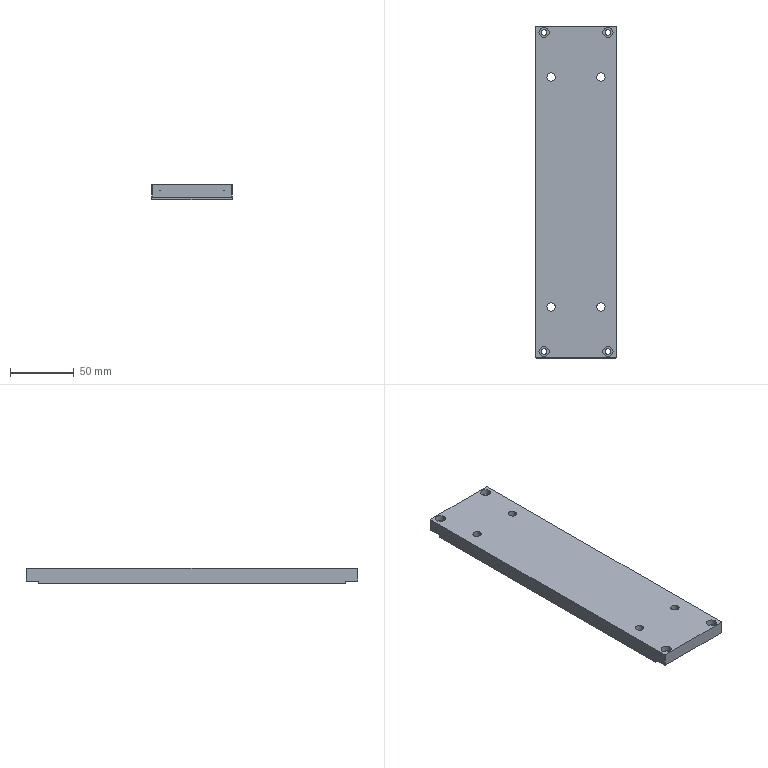Part | STEP file | 2031 Base bottom plate | 1 solid | 42 faces | box 63 x 260 x 12 mm | volume 191174 mm3 | cylinder 24 | plane 18 | commonest cylinder face diameters 4.5 x8 6.5 x8 8 x8